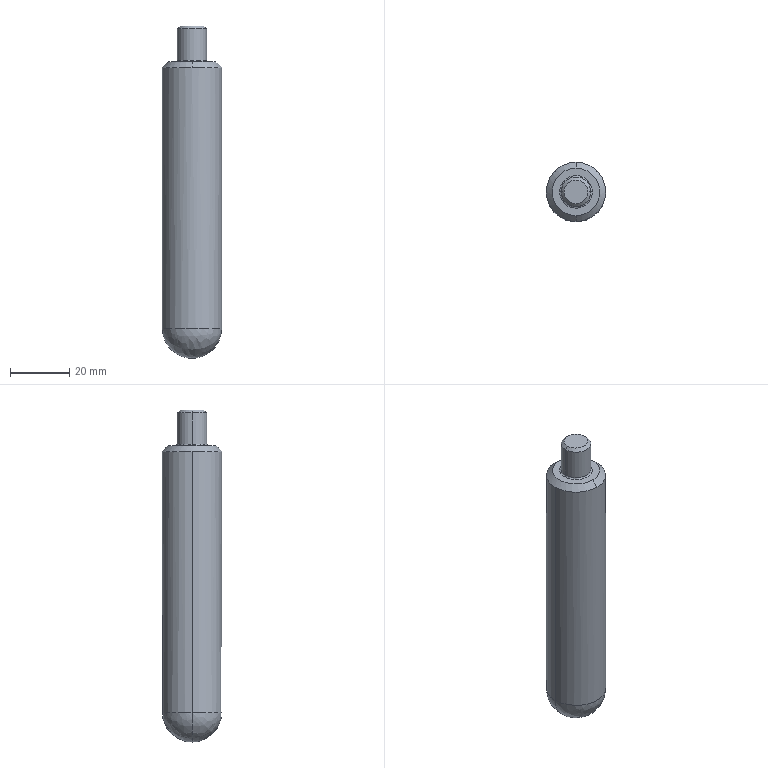Part | STEP file | Handle new | 1 solid | 14 faces | box 20 x 20 x 112 mm | volume 31180 mm3 | spline 4 | cylinder 4 | cone 4 | plane 2 | commonest cylinder face diameters 10 x2 20 x2